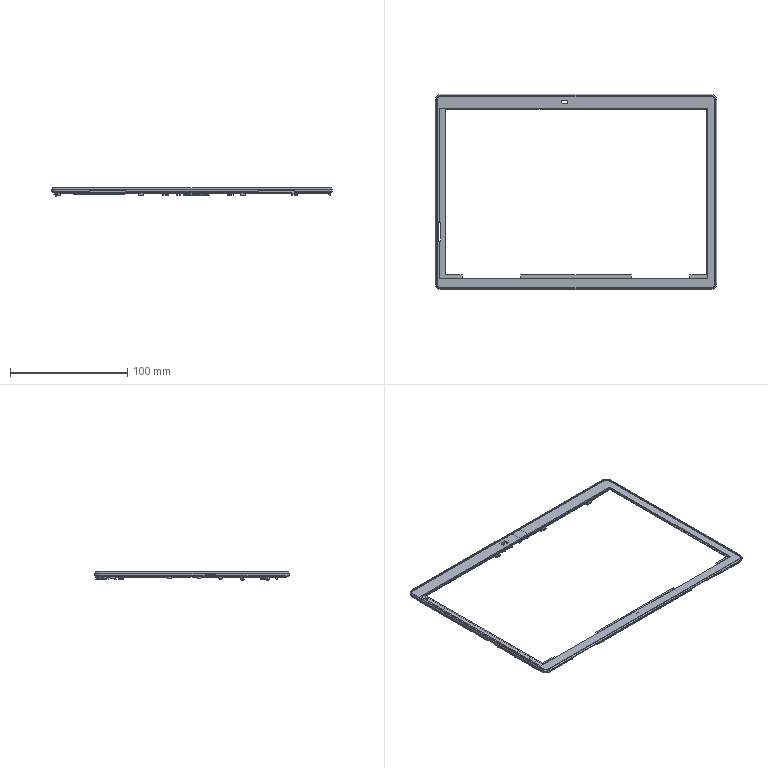Part | Creo | 1 solid | 617 faces | box 239.74 x 166.74 x 6.94 mm | volume 15309 mm3 | plane 476 | cylinder 97 | cone 18 | torus 16 | spline 10 | commonest cylinder face diameters 1.1 x28 3 x10 1.3 x8 3.3 x8 1.2 x7 2.2 x4